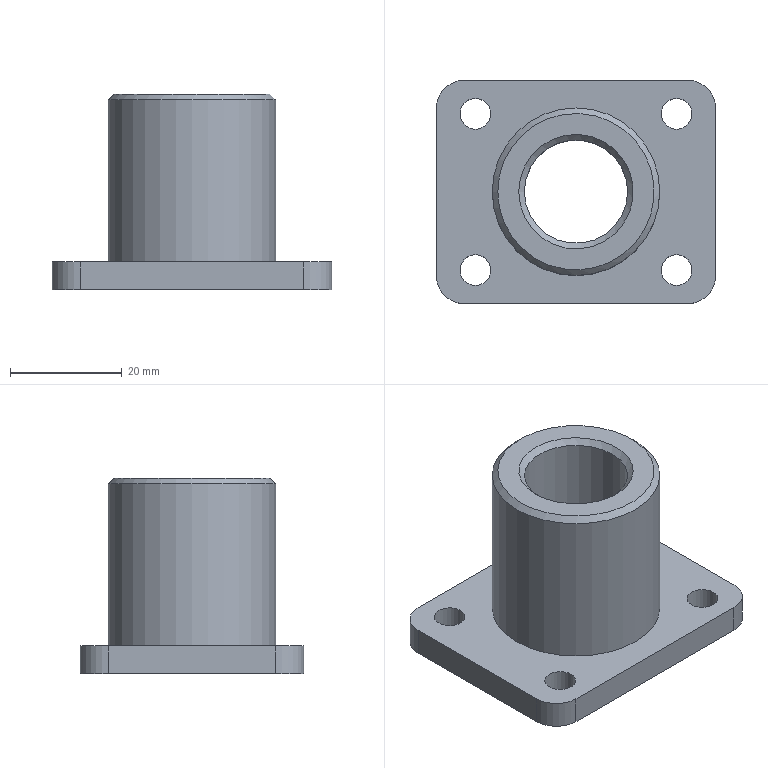Part | NX | 1 solid | 20 faces | box 50 x 40 x 35 mm | volume 21109 mm3 | cylinder 10 | plane 7 | cone 3 | commonest cylinder face diameters 5.5 x4 10 x4 18.5 x1 30 x1
STEP:
#1=CARTESIAN_POINT('',(201.752,213.797,-5.));
#2=VERTEX_POINT('',#1);
#3=CARTESIAN_POINT('',(191.502,213.797,-5.));
#4=DIRECTION('',(0.,0.,1.));
#5=DIRECTION('',(1.,0.,0.));
#6=AXIS2_PLACEMENT_3D('',#3,#4,#5);
#7=CIRCLE('',#6,10.25);
#8=EDGE_CURVE('',#2,#2,#7,.T.);
#9=ORIENTED_EDGE('',*,*,#8,.T.);
#10=EDGE_LOOP('',(#9));
#11=FACE_BOUND('',#10,.T.);
#12=CARTESIAN_POINT('',(176.252,199.797,-5.));
#13=VERTEX_POINT('',#12);
#14=CARTESIAN_POINT('',(173.502,199.797,-5.));
#15=DIRECTION('',(0.,0.,1.));
#16=DIRECTION('',(1.,0.,0.));
#17=AXIS2_PLACEMENT_3D('',#14,#15,#16);
#18=CIRCLE('',#17,2.75);
#19=EDGE_CURVE('',#13,#13,#18,.T.);
#20=ORIENTED_EDGE('',*,*,#19,.T.);
#21=EDGE_LOOP('',(#20));
#22=FACE_BOUND('',#21,.T.);
#23=CARTESIAN_POINT('',(212.252,199.797,-5.));
#24=VERTEX_POINT('',#23);
#25=CARTESIAN_POINT('',(209.502,199.797,-5.));
#26=DIRECTION('',(0.,0.,1.));
#27=DIRECTION('',(1.,0.,0.));
#28=AXIS2_PLACEMENT_3D('',#25,#26,#27);
#29=CIRCLE('',#28,2.75);
#30=EDGE_CURVE('',#24,#24,#29,.T.);
#31=ORIENTED_EDGE('',*,*,#30,.T.);
#32=EDGE_LOOP('',(#31));
#33=FACE_BOUND('',#32,.T.);
#34=CARTESIAN_POINT('',(212.252,227.797,-5.));
#35=VERTEX_POINT('',#34);
#36=CARTESIAN_POINT('',(209.502,227.797,-5.));
#37=DIRECTION('',(0.,0.,1.));
#38=DIRECTION('',(1.,0.,0.));
#39=AXIS2_PLACEMENT_3D('',#36,#37,#38);
#40=CIRCLE('',#39,2.75);
#41=EDGE_CURVE('',#35,#35,#40,.T.);
#42=ORIENTED_EDGE('',*,*,#41,.T.);
#43=EDGE_LOOP('',(#42));
#44=FACE_BOUND('',#43,.T.);
#45=CARTESIAN_POINT('',(171.502,233.797,-5.));
#46=VERTEX_POINT('',#45);
#47=CARTESIAN_POINT('',(166.502,228.797,-5.));
#48=VERTEX_POINT('',#47);
#49=CARTESIAN_POINT('',(171.502,228.797,-5.));
#50=DIRECTION('',(0.,0.,1.));
#51=DIRECTION('',(1.,0.,0.));
#52=AXIS2_PLACEMENT_3D('',#49,#50,#51);
#53=CIRCLE('',#52,5.);
#54=EDGE_CURVE('',#46,#48,#53,.T.);
#55=ORIENTED_EDGE('',*,*,#54,.F.);
#56=CARTESIAN_POINT('',(211.502,233.797,-5.));
#57=VERTEX_POINT('',#56);
#58=CARTESIAN_POINT('',(211.502,233.797,-5.));
#59=DIRECTION('',(-1.,0.,0.));
#60=VECTOR('',#59,1000.);
#61=LINE('',#58,#60);
#62=EDGE_CURVE('',#57,#46,#61,.T.);
#63=ORIENTED_EDGE('',*,*,#62,.F.);
#64=CARTESIAN_POINT('',(216.502,228.797,-5.));
#65=VERTEX_POINT('',#64);
#66=CARTESIAN_POINT('',(211.502,228.797,-5.));
#67=DIRECTION('',(0.,0.,1.));
#68=DIRECTION('',(1.,0.,0.));
#69=AXIS2_PLACEMENT_3D('',#66,#67,#68);
#70=CIRCLE('',#69,5.);
#71=EDGE_CURVE('',#65,#57,#70,.T.);
#72=ORIENTED_EDGE('',*,*,#71,.F.);
#73=CARTESIAN_POINT('',(216.502,198.797,-5.));
#74=VERTEX_POINT('',#73);
#75=CARTESIAN_POINT('',(216.502,198.797,-5.));
#76=DIRECTION('',(0.,1.,0.));
#77=VECTOR('',#76,1000.);
#78=LINE('',#75,#77);
#79=EDGE_CURVE('',#74,#65,#78,.T.);
#80=ORIENTED_EDGE('',*,*,#79,.F.);
#81=CARTESIAN_POINT('',(211.502,193.797,-5.));
#82=VERTEX_POINT('',#81);
#83=CARTESIAN_POINT('',(211.502,198.797,-5.));
#84=DIRECTION('',(0.,0.,1.));
#85=DIRECTION('',(1.,0.,0.));
#86=AXIS2_PLACEMENT_3D('',#83,#84,#85);
#87=CIRCLE('',#86,5.);
#88=EDGE_CURVE('',#82,#74,#87,.T.);
#89=ORIENTED_EDGE('',*,*,#88,.F.);
#90=CARTESIAN_POINT('',(171.502,193.797,-5.));
#91=VERTEX_POINT('',#90);
#92=CARTESIAN_POINT('',(171.502,193.797,-5.));
#93=DIRECTION('',(1.,0.,0.));
#94=VECTOR('',#93,1000.);
#95=LINE('',#92,#94);
#96=EDGE_CURVE('',#91,#82,#95,.T.);
#97=ORIENTED_EDGE('',*,*,#96,.F.);
#98=CARTESIAN_POINT('',(166.502,198.797,-5.));
#99=VERTEX_POINT('',#98);
#100=CARTESIAN_POINT('',(171.502,198.797,-5.));
#101=DIRECTION('',(0.,0.,1.));
#102=DIRECTION('',(1.,0.,0.));
#103=AXIS2_PLACEMENT_3D('',#100,#101,#102);
#104=CIRCLE('',#103,5.);
#105=EDGE_CURVE('',#99,#91,#104,.T.);
#106=ORIENTED_EDGE('',*,*,#105,.F.);
#107=CARTESIAN_POINT('',(166.502,228.797,-5.));
#108=DIRECTION('',(0.,-1.,0.));
#109=VECTOR('',#108,1000.);
#110=LINE('',#107,#109);
#111=EDGE_CURVE('',#48,#99,#110,.T.);
#112=ORIENTED_EDGE('',*,*,#111,.F.);
#113=EDGE_LOOP('',(#55,#63,#72,#80,#89,#97,#106,#112));
#114=FACE_BOUND('',#113,.T.);
#115=CARTESIAN_POINT('',(176.252,227.797,-5.));
#116=VERTEX_POINT('',#115);
#117=CARTESIAN_POINT('',(173.502,227.797,-5.));
#118=DIRECTION('',(0.,0.,-1.));
#119=DIRECTION('',(1.,0.,0.));
#120=AXIS2_PLACEMENT_3D('',#117,#118,#119);
#121=CIRCLE('',#120,2.75);
#122=EDGE_CURVE('',#116,#116,#121,.T.);
#123=ORIENTED_EDGE('',*,*,#122,.F.);
#124=EDGE_LOOP('',(#123));
#125=FACE_BOUND('',#124,.T.);
#126=CARTESIAN_POINT('',(171.502,228.797,-5.));
#127=DIRECTION('',(0.,0.,1.));
#128=DIRECTION('',(1.,0.,0.));
#129=AXIS2_PLACEMENT_3D('',#126,#127,#128);
#130=PLANE('',#129);
#131=ADVANCED_FACE('',(#11,#22,#33,#44,#114,#125),#130,.F.);
#132=CARTESIAN_POINT('',(206.502,213.797,0.));
#133=VERTEX_POINT('',#132);
#134=CARTESIAN_POINT('',(191.502,213.797,0.));
#135=DIRECTION('',(0.,0.,-1.));
#136=DIRECTION('',(1.,0.,0.));
#137=AXIS2_PLACEMENT_3D('',#134,#135,#136);
#138=CIRCLE('',#137,15.);
#139=EDGE_CURVE('',#133,#133,#138,.T.);
#140=ORIENTED_EDGE('',*,*,#139,.T.);
#141=EDGE_LOOP('',(#140));
#142=FACE_BOUND('',#141,.T.);
#143=CARTESIAN_POINT('',(171.502,233.797,0.));
#144=VERTEX_POINT('',#143);
#145=CARTESIAN_POINT('',(166.502,228.797,0.));
#146=VERTEX_POINT('',#145);
#147=CARTESIAN_POINT('',(171.502,228.797,0.));
#148=DIRECTION('',(0.,0.,1.));
#149=DIRECTION('',(1.,0.,0.));
#150=AXIS2_PLACEMENT_3D('',#147,#148,#149);
#151=CIRCLE('',#150,5.);
#152=EDGE_CURVE('',#144,#146,#151,.T.);
#153=ORIENTED_EDGE('',*,*,#152,.T.);
#154=CARTESIAN_POINT('',(166.502,198.797,0.));
#155=VERTEX_POINT('',#154);
#156=CARTESIAN_POINT('',(166.502,228.797,0.));
#157=DIRECTION('',(0.,-1.,0.));
#158=VECTOR('',#157,1000.);
#159=LINE('',#156,#158);
#160=EDGE_CURVE('',#146,#155,#159,.T.);
#161=ORIENTED_EDGE('',*,*,#160,.T.);
#162=CARTESIAN_POINT('',(171.502,193.797,0.));
#163=VERTEX_POINT('',#162);
#164=CARTESIAN_POINT('',(171.502,198.797,0.));
#165=DIRECTION('',(0.,0.,1.));
#166=DIRECTION('',(1.,0.,0.));
#167=AXIS2_PLACEMENT_3D('',#164,#165,#166);
#168=CIRCLE('',#167,5.);
#169=EDGE_CURVE('',#155,#163,#168,.T.);
#170=ORIENTED_EDGE('',*,*,#169,.T.);
#171=CARTESIAN_POINT('',(211.502,193.797,0.));
#172=VERTEX_POINT('',#171);
#173=CARTESIAN_POINT('',(171.502,193.797,0.));
#174=DIRECTION('',(1.,0.,0.));
#175=VECTOR('',#174,1000.);
#176=LINE('',#173,#175);
#177=EDGE_CURVE('',#163,#172,#176,.T.);
#178=ORIENTED_EDGE('',*,*,#177,.T.);
#179=CARTESIAN_POINT('',(216.502,198.797,0.));
#180=VERTEX_POINT('',#179);
#181=CARTESIAN_POINT('',(211.502,198.797,0.));
#182=DIRECTION('',(0.,0.,1.));
#183=DIRECTION('',(1.,0.,0.));
#184=AXIS2_PLACEMENT_3D('',#181,#182,#183);
#185=CIRCLE('',#184,5.);
#186=EDGE_CURVE('',#172,#180,#185,.T.);
#187=ORIENTED_EDGE('',*,*,#186,.T.);
#188=CARTESIAN_POINT('',(216.502,228.797,0.));
#189=VERTEX_POINT('',#188);
#190=CARTESIAN_POINT('',(216.502,198.797,0.));
#191=DIRECTION('',(0.,1.,0.));
#192=VECTOR('',#191,1000.);
#193=LINE('',#190,#192);
#194=EDGE_CURVE('',#180,#189,#193,.T.);
#195=ORIENTED_EDGE('',*,*,#194,.T.);
#196=CARTESIAN_POINT('',(211.502,233.797,0.));
#197=VERTEX_POINT('',#196);
#198=CARTESIAN_POINT('',(211.502,228.797,0.));
#199=DIRECTION('',(0.,0.,1.));
#200=DIRECTION('',(1.,0.,0.));
#201=AXIS2_PLACEMENT_3D('',#198,#199,#200);
#202=CIRCLE('',#201,5.);
#203=EDGE_CURVE('',#189,#197,#202,.T.);
#204=ORIENTED_EDGE('',*,*,#203,.T.);
#205=CARTESIAN_POINT('',(211.502,233.797,0.));
#206=DIRECTION('',(-1.,0.,0.));
#207=VECTOR('',#206,1000.);
#208=LINE('',#205,#207);
#209=EDGE_CURVE('',#197,#144,#208,.T.);
#210=ORIENTED_EDGE('',*,*,#209,.T.);
#211=EDGE_LOOP('',(#153,#161,#170,#178,#187,#195,#204,#210));
#212=FACE_BOUND('',#211,.T.);
#213=CARTESIAN_POINT('',(212.252,227.797,0.));
#214=VERTEX_POINT('',#213);
#215=CARTESIAN_POINT('',(209.502,227.797,0.));
#216=DIRECTION('',(0.,0.,1.));
#217=DIRECTION('',(1.,0.,0.));
#218=AXIS2_PLACEMENT_3D('',#215,#216,#217);
#219=CIRCLE('',#218,2.75);
#220=EDGE_CURVE('',#214,#214,#219,.T.);
#221=ORIENTED_EDGE('',*,*,#220,.F.);
#222=EDGE_LOOP('',(#221));
#223=FACE_BOUND('',#222,.T.);
#224=CARTESIAN_POINT('',(212.252,199.797,0.));
#225=VERTEX_POINT('',#224);
#226=CARTESIAN_POINT('',(209.502,199.797,0.));
#227=DIRECTION('',(0.,0.,1.));
#228=DIRECTION('',(1.,0.,0.));
#229=AXIS2_PLACEMENT_3D('',#226,#227,#228);
#230=CIRCLE('',#229,2.75);
#231=EDGE_CURVE('',#225,#225,#230,.T.);
#232=ORIENTED_EDGE('',*,*,#231,.F.);
#233=EDGE_LOOP('',(#232));
#234=FACE_BOUND('',#233,.T.);
#235=CARTESIAN_POINT('',(176.252,199.797,0.));
#236=VERTEX_POINT('',#235);
#237=CARTESIAN_POINT('',(173.502,199.797,0.));
#238=DIRECTION('',(0.,0.,1.));
#239=DIRECTION('',(1.,0.,0.));
#240=AXIS2_PLACEMENT_3D('',#237,#238,#239);
#241=CIRCLE('',#240,2.75);
#242=EDGE_CURVE('',#236,#236,#241,.T.);
#243=ORIENTED_EDGE('',*,*,#242,.F.);
#244=EDGE_LOOP('',(#243));
#245=FACE_BOUND('',#244,.T.);
#246=CARTESIAN_POINT('',(176.252,227.797,0.));
#247=VERTEX_POINT('',#246);
#248=CARTESIAN_POINT('',(173.502,227.797,0.));
#249=DIRECTION('',(0.,0.,-1.));
#250=DIRECTION('',(1.,0.,0.));
#251=AXIS2_PLACEMENT_3D('',#248,#249,#250);
#252=CIRCLE('',#251,2.75);
#253=EDGE_CURVE('',#247,#247,#252,.T.);
#254=ORIENTED_EDGE('',*,*,#253,.T.);
#255=EDGE_LOOP('',(#254));
#256=FACE_BOUND('',#255,.T.);
#257=CARTESIAN_POINT('',(171.502,228.797,0.));
#258=DIRECTION('',(0.,0.,1.));
#259=DIRECTION('',(1.,0.,0.));
#260=AXIS2_PLACEMENT_3D('',#257,#258,#259);
#261=PLANE('',#260);
#262=ADVANCED_FACE('',(#142,#212,#223,#234,#245,#256),#261,.T.);
#263=ORIENTED_EDGE('',*,*,#152,.F.);
#264=CARTESIAN_POINT('',(171.502,233.797,-5.));
#265=DIRECTION('',(0.,0.,1.));
#266=VECTOR('',#265,1000.);
#267=LINE('',#264,#266);
#268=EDGE_CURVE('',#46,#144,#267,.T.);
#269=ORIENTED_EDGE('',*,*,#268,.F.);
#270=ORIENTED_EDGE('',*,*,#54,.T.);
#271=CARTESIAN_POINT('',(166.502,228.797,-5.));
#272=DIRECTION('',(0.,0.,1.));
#273=VECTOR('',#272,1000.);
#274=LINE('',#271,#273);
#275=EDGE_CURVE('',#48,#146,#274,.T.);
#276=ORIENTED_EDGE('',*,*,#275,.T.);
#277=EDGE_LOOP('',(#263,#269,#270,#276));
#278=FACE_BOUND('',#277,.T.);
#279=CARTESIAN_POINT('',(171.502,228.797,-5.));
#280=DIRECTION('',(0.,0.,1.));
#281=DIRECTION('',(1.,0.,0.));
#282=AXIS2_PLACEMENT_3D('',#279,#280,#281);
#283=CYLINDRICAL_SURFACE('',#282,5.);
#284=ADVANCED_FACE('',(#278),#283,.T.);
#285=ORIENTED_EDGE('',*,*,#160,.F.);
#286=ORIENTED_EDGE('',*,*,#275,.F.);
#287=ORIENTED_EDGE('',*,*,#111,.T.);
#288=CARTESIAN_POINT('',(166.502,198.797,-5.));
#289=DIRECTION('',(0.,0.,1.));
#290=VECTOR('',#289,1000.);
#291=LINE('',#288,#290);
#292=EDGE_CURVE('',#99,#155,#291,.T.);
#293=ORIENTED_EDGE('',*,*,#292,.T.);
#294=EDGE_LOOP('',(#285,#286,#287,#293));
#295=FACE_BOUND('',#294,.T.);
#296=CARTESIAN_POINT('',(166.502,228.797,-5.));
#297=DIRECTION('',(-1.,0.,0.));
#298=DIRECTION('',(0.,0.,1.));
#299=AXIS2_PLACEMENT_3D('',#296,#297,#298);
#300=PLANE('',#299);
#301=ADVANCED_FACE('',(#295),#300,.T.);
#302=ORIENTED_EDGE('',*,*,#169,.F.);
#303=ORIENTED_EDGE('',*,*,#292,.F.);
#304=ORIENTED_EDGE('',*,*,#105,.T.);
#305=CARTESIAN_POINT('',(171.502,193.797,-5.));
#306=DIRECTION('',(0.,0.,1.));
#307=VECTOR('',#306,1000.);
#308=LINE('',#305,#307);
#309=EDGE_CURVE('',#91,#163,#308,.T.);
#310=ORIENTED_EDGE('',*,*,#309,.T.);
#311=EDGE_LOOP('',(#302,#303,#304,#310));
#312=FACE_BOUND('',#311,.T.);
#313=CARTESIAN_POINT('',(171.502,198.797,-5.));
#314=DIRECTION('',(0.,0.,1.));
#315=DIRECTION('',(1.,0.,0.));
#316=AXIS2_PLACEMENT_3D('',#313,#314,#315);
#317=CYLINDRICAL_SURFACE('',#316,5.);
#318=ADVANCED_FACE('',(#312),#317,.T.);
#319=ORIENTED_EDGE('',*,*,#177,.F.);
#320=ORIENTED_EDGE('',*,*,#309,.F.);
#321=ORIENTED_EDGE('',*,*,#96,.T.);
#322=CARTESIAN_POINT('',(211.502,193.797,-5.));
#323=DIRECTION('',(0.,0.,1.));
#324=VECTOR('',#323,1000.);
#325=LINE('',#322,#324);
#326=EDGE_CURVE('',#82,#172,#325,.T.);
#327=ORIENTED_EDGE('',*,*,#326,.T.);
#328=EDGE_LOOP('',(#319,#320,#321,#327));
#329=FACE_BOUND('',#328,.T.);
#330=CARTESIAN_POINT('',(171.502,193.797,-5.));
#331=DIRECTION('',(0.,-1.,0.));
#332=DIRECTION('',(0.,0.,-1.));
#333=AXIS2_PLACEMENT_3D('',#330,#331,#332);
#334=PLANE('',#333);
#335=ADVANCED_FACE('',(#329),#334,.T.);
#336=ORIENTED_EDGE('',*,*,#186,.F.);
#337=ORIENTED_EDGE('',*,*,#326,.F.);
#338=ORIENTED_EDGE('',*,*,#88,.T.);
#339=CARTESIAN_POINT('',(216.502,198.797,-5.));
#340=DIRECTION('',(0.,0.,1.));
#341=VECTOR('',#340,1000.);
#342=LINE('',#339,#341);
#343=EDGE_CURVE('',#74,#180,#342,.T.);
#344=ORIENTED_EDGE('',*,*,#343,.T.);
#345=EDGE_LOOP('',(#336,#337,#338,#344));
#346=FACE_BOUND('',#345,.T.);
#347=CARTESIAN_POINT('',(211.502,198.797,-5.));
#348=DIRECTION('',(0.,0.,1.));
#349=DIRECTION('',(1.,0.,0.));
#350=AXIS2_PLACEMENT_3D('',#347,#348,#349);
#351=CYLINDRICAL_SURFACE('',#350,5.);
#352=ADVANCED_FACE('',(#346),#351,.T.);
#353=ORIENTED_EDGE('',*,*,#194,.F.);
#354=ORIENTED_EDGE('',*,*,#343,.F.);
#355=ORIENTED_EDGE('',*,*,#79,.T.);
#356=CARTESIAN_POINT('',(216.502,228.797,-5.));
#357=DIRECTION('',(0.,0.,1.));
#358=VECTOR('',#357,1000.);
#359=LINE('',#356,#358);
#360=EDGE_CURVE('',#65,#189,#359,.T.);
#361=ORIENTED_EDGE('',*,*,#360,.T.);
#362=EDGE_LOOP('',(#353,#354,#355,#361));
#363=FACE_BOUND('',#362,.T.);
#364=CARTESIAN_POINT('',(216.502,198.797,-5.));
#365=DIRECTION('',(1.,0.,0.));
#366=DIRECTION('',(0.,0.,-1.));
#367=AXIS2_PLACEMENT_3D('',#364,#365,#366);
#368=PLANE('',#367);
#369=ADVANCED_FACE('',(#363),#368,.T.);
#370=ORIENTED_EDGE('',*,*,#203,.F.);
#371=ORIENTED_EDGE('',*,*,#360,.F.);
#372=ORIENTED_EDGE('',*,*,#71,.T.);
#373=CARTESIAN_POINT('',(211.502,233.797,-5.));
#374=DIRECTION('',(0.,0.,1.));
#375=VECTOR('',#374,1000.);
#376=LINE('',#373,#375);
#377=EDGE_CURVE('',#57,#197,#376,.T.);
#378=ORIENTED_EDGE('',*,*,#377,.T.);
#379=EDGE_LOOP('',(#370,#371,#372,#378));
#380=FACE_BOUND('',#379,.T.);
#381=CARTESIAN_POINT('',(211.502,228.797,-5.));
#382=DIRECTION('',(0.,0.,1.));
#383=DIRECTION('',(1.,0.,0.));
#384=AXIS2_PLACEMENT_3D('',#381,#382,#383);
#385=CYLINDRICAL_SURFACE('',#384,5.);
#386=ADVANCED_FACE('',(#380),#385,.T.);
#387=ORIENTED_EDGE('',*,*,#209,.F.);
#388=ORIENTED_EDGE('',*,*,#377,.F.);
#389=ORIENTED_EDGE('',*,*,#62,.T.);
#390=ORIENTED_EDGE('',*,*,#268,.T.);
#391=EDGE_LOOP('',(#387,#388,#389,#390));
#392=FACE_BOUND('',#391,.T.);
#393=CARTESIAN_POINT('',(211.502,233.797,-5.));
#394=DIRECTION('',(0.,1.,0.));
#395=DIRECTION('',(0.,0.,1.));
#396=AXIS2_PLACEMENT_3D('',#393,#394,#395);
#397=PLANE('',#396);
#398=ADVANCED_FACE('',(#392),#397,.T.);
#399=ORIENTED_EDGE('',*,*,#41,.F.);
#400=EDGE_LOOP('',(#399));
#401=FACE_BOUND('',#400,.T.);
#402=ORIENTED_EDGE('',*,*,#220,.T.);
#403=EDGE_LOOP('',(#402));
#404=FACE_BOUND('',#403,.T.);
#405=CARTESIAN_POINT('',(209.502,227.797,-5.));
#406=DIRECTION('',(0.,0.,1.));
#407=DIRECTION('',(1.,0.,0.));
#408=AXIS2_PLACEMENT_3D('',#405,#406,#407);
#409=CYLINDRICAL_SURFACE('',#408,2.75);
#410=ADVANCED_FACE('',(#401,#404),#409,.F.);
#411=ORIENTED_EDGE('',*,*,#30,.F.);
#412=EDGE_LOOP('',(#411));
#413=FACE_BOUND('',#412,.T.);
#414=ORIENTED_EDGE('',*,*,#231,.T.);
#415=EDGE_LOOP('',(#414));
#416=FACE_BOUND('',#415,.T.);
#417=CARTESIAN_POINT('',(209.502,199.797,-5.));
#418=DIRECTION('',(0.,0.,1.));
#419=DIRECTION('',(1.,0.,0.));
#420=AXIS2_PLACEMENT_3D('',#417,#418,#419);
#421=CYLINDRICAL_SURFACE('',#420,2.75);
#422=ADVANCED_FACE('',(#413,#416),#421,.F.);
#423=ORIENTED_EDGE('',*,*,#19,.F.);
#424=EDGE_LOOP('',(#423));
#425=FACE_BOUND('',#424,.T.);
#426=ORIENTED_EDGE('',*,*,#242,.T.);
#427=EDGE_LOOP('',(#426));
#428=FACE_BOUND('',#427,.T.);
#429=CARTESIAN_POINT('',(173.502,199.797,-5.));
#430=DIRECTION('',(0.,0.,1.));
#431=DIRECTION('',(1.,0.,0.));
#432=AXIS2_PLACEMENT_3D('',#429,#430,#431);
#433=CYLINDRICAL_SURFACE('',#432,2.75);
#434=ADVANCED_FACE('',(#425,#428),#433,.F.);
#435=ORIENTED_EDGE('',*,*,#122,.T.);
#436=EDGE_LOOP('',(#435));
#437=FACE_BOUND('',#436,.T.);
#438=ORIENTED_EDGE('',*,*,#253,.F.);
#439=EDGE_LOOP('',(#438));
#440=FACE_BOUND('',#439,.T.);
#441=CARTESIAN_POINT('',(173.502,227.797,-5.));
#442=DIRECTION('',(0.,0.,1.));
#443=DIRECTION('',(1.,0.,0.));
#444=AXIS2_PLACEMENT_3D('',#441,#442,#443);
#445=CYLINDRICAL_SURFACE('',#444,2.75);
#446=ADVANCED_FACE('',(#437,#440),#445,.F.);
#447=CARTESIAN_POINT('',(176.502,213.797,29.));
#448=VERTEX_POINT('',#447);
#449=CARTESIAN_POINT('',(191.502,213.797,29.));
#450=DIRECTION('',(0.,0.,-1.));
#451=DIRECTION('',(-1.,0.,0.));
#452=AXIS2_PLACEMENT_3D('',#449,#450,#451);
#453=CIRCLE('',#452,15.);
#454=EDGE_CURVE('',#448,#448,#453,.T.);
#455=ORIENTED_EDGE('',*,*,#454,.T.);
#456=EDGE_LOOP('',(#455));
#457=FACE_BOUND('',#456,.T.);
#458=ORIENTED_EDGE('',*,*,#139,.F.);
#459=EDGE_LOOP('',(#458));
#460=FACE_BOUND('',#459,.T.);
#461=CARTESIAN_POINT('',(191.502,213.797,30.));
#462=DIRECTION('',(0.,0.,-1.));
#463=DIRECTION('',(-1.,0.,0.));
#464=AXIS2_PLACEMENT_3D('',#461,#462,#463);
#465=CYLINDRICAL_SURFACE('',#464,15.);
#466=ADVANCED_FACE('',(#457,#460),#465,.T.);
#467=CARTESIAN_POINT('',(181.252,213.797,30.));
#468=VERTEX_POINT('',#467);
#469=CARTESIAN_POINT('',(191.502,213.797,30.));
#470=DIRECTION('',(0.,0.,-1.));
#471=DIRECTION('',(-1.,0.,0.));
#472=AXIS2_PLACEMENT_3D('',#469,#470,#471);
#473=CIRCLE('',#472,10.25);
#474=EDGE_CURVE('',#468,#468,#473,.T.);
#475=ORIENTED_EDGE('',*,*,#474,.T.);
#476=EDGE_LOOP('',(#475));
#477=FACE_BOUND('',#476,.T.);
#478=CARTESIAN_POINT('',(177.502,213.797,30.));
#479=VERTEX_POINT('',#478);
#480=CARTESIAN_POINT('',(191.502,213.797,30.));
#481=DIRECTION('',(0.,0.,-1.));
#482=DIRECTION('',(-1.,0.,0.));
#483=AXIS2_PLACEMENT_3D('',#480,#481,#482);
#484=CIRCLE('',#483,14.);
#485=EDGE_CURVE('',#479,#479,#484,.F.);
#486=ORIENTED_EDGE('',*,*,#485,.T.);
#487=EDGE_LOOP('',(#486));
#488=FACE_BOUND('',#487,.T.);
#489=CARTESIAN_POINT('',(191.502,213.797,30.));
#490=DIRECTION('',(0.,0.,-1.));
#491=DIRECTION('',(-1.,0.,0.));
#492=AXIS2_PLACEMENT_3D('',#489,#490,#491);
#493=PLANE('',#492);
#494=ADVANCED_FACE('',(#477,#488),#493,.F.);
#495=CARTESIAN_POINT('',(182.252,213.797,-4.));
#496=VERTEX_POINT('',#495);
#497=CARTESIAN_POINT('',(191.502,213.797,-4.));
#498=DIRECTION('',(0.,0.,-1.));
#499=DIRECTION('',(-1.,0.,0.));
#500=AXIS2_PLACEMENT_3D('',#497,#498,#499);
#501=CIRCLE('',#500,9.25);
#502=EDGE_CURVE('',#496,#496,#501,.T.);
#503=ORIENTED_EDGE('',*,*,#502,.T.);
#504=EDGE_LOOP('',(#503));
#505=FACE_BOUND('',#504,.T.);
#506=CARTESIAN_POINT('',(200.752,213.797,29.));
#507=VERTEX_POINT('',#506);
#508=CARTESIAN_POINT('',(191.502,213.797,29.));
#509=DIRECTION('',(0.,0.,1.));
#510=DIRECTION('',(1.,0.,0.));
#511=AXIS2_PLACEMENT_3D('',#508,#509,#510);
#512=CIRCLE('',#511,9.25);
#513=EDGE_CURVE('',#507,#507,#512,.T.);
#514=ORIENTED_EDGE('',*,*,#513,.T.);
#515=EDGE_LOOP('',(#514));
#516=FACE_BOUND('',#515,.T.);
#517=CARTESIAN_POINT('',(191.502,213.797,30.));
#518=DIRECTION('',(0.,0.,-1.));
#519=DIRECTION('',(-1.,0.,0.));
#520=AXIS2_PLACEMENT_3D('',#517,#518,#519);
#521=CYLINDRICAL_SURFACE('',#520,9.25);
#522=ADVANCED_FACE('',(#505,#516),#521,.F.);
#523=ORIENTED_EDGE('',*,*,#485,.F.);
#524=EDGE_LOOP('',(#523));
#525=FACE_BOUND('',#524,.T.);
#526=ORIENTED_EDGE('',*,*,#454,.F.);
#527=EDGE_LOOP('',(#526));
#528=FACE_BOUND('',#527,.T.);
#529=CARTESIAN_POINT('',(191.502,213.797,29.));
#530=DIRECTION('',(0.,0.,-1.));
#531=DIRECTION('',(-1.,0.,0.));
#532=AXIS2_PLACEMENT_3D('',#529,#530,#531);
#533=CONICAL_SURFACE('',#532,15.,0.7854);
#534=ADVANCED_FACE('',(#525,#528),#533,.T.);
#535=ORIENTED_EDGE('',*,*,#502,.F.);
#536=EDGE_LOOP('',(#535));
#537=FACE_BOUND('',#536,.T.);
#538=ORIENTED_EDGE('',*,*,#8,.F.);
#539=EDGE_LOOP('',(#538));
#540=FACE_BOUND('',#539,.T.);
#541=CARTESIAN_POINT('',(191.502,213.797,-5.));
#542=DIRECTION('',(0.,0.,-1.));
#543=DIRECTION('',(-1.,0.,0.));
#544=AXIS2_PLACEMENT_3D('',#541,#542,#543);
#545=CONICAL_SURFACE('',#544,10.25,0.7854);
#546=ADVANCED_FACE('',(#537,#540),#545,.F.);
#547=ORIENTED_EDGE('',*,*,#513,.F.);
#548=EDGE_LOOP('',(#547));
#549=FACE_BOUND('',#548,.T.);
#550=ORIENTED_EDGE('',*,*,#474,.F.);
#551=EDGE_LOOP('',(#550));
#552=FACE_BOUND('',#551,.T.);
#553=CARTESIAN_POINT('',(191.502,213.797,30.));
#554=DIRECTION('',(0.,0.,1.));
#555=DIRECTION('',(1.,0.,0.));
#556=AXIS2_PLACEMENT_3D('',#553,#554,#555);
#557=CONICAL_SURFACE('',#556,10.25,0.7854);
#558=ADVANCED_FACE('',(#549,#552),#557,.F.);
#559=CLOSED_SHELL('',(#131,#262,#284,#301,#318,#335,#352,#369,#386,#398,#410,#422,#434,#446,#466,#494,#522,#534,#546,#558));
#560=MANIFOLD_SOLID_BREP('',#559);
#561=(LENGTH_UNIT()NAMED_UNIT(*)SI_UNIT(.MILLI.,.METRE.));
#562=UNCERTAINTY_MEASURE_WITH_UNIT(LENGTH_MEASURE(0.00001),#561,'','');
#563=(NAMED_UNIT(*)PLANE_ANGLE_UNIT()SI_UNIT($,.RADIAN.));
#564=(NAMED_UNIT(*)SI_UNIT($,.STERADIAN.)SOLID_ANGLE_UNIT());
#565=(GEOMETRIC_REPRESENTATION_CONTEXT(3)GLOBAL_UNCERTAINTY_ASSIGNED_CONTEXT((#562))GLOBAL_UNIT_ASSIGNED_CONTEXT((#561,#563,#564))REPRESENTATION_CONTEXT('',''));
#566=ADVANCED_BREP_SHAPE_REPRESENTATION('',(#560),#565);